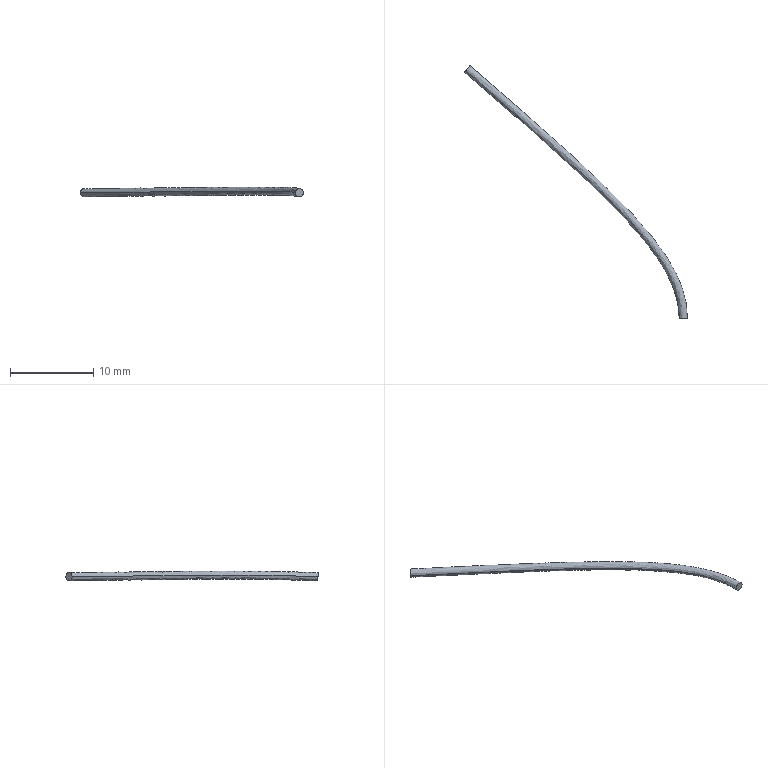Part | NX | features BREP 1 | 1 solid | 4 faces | box 26.795 x 30.33 x 1.202 mm | volume 31.795 mm3 | plane 2 | spline 2
STEP:
#1=CARTESIAN_POINT('',(-445.099,275.62,219.465));
#2=VERTEX_POINT('',#1);
#3=CARTESIAN_POINT('',(-444.445,276.376,219.465));
#4=VERTEX_POINT('',#3);
#5=CARTESIAN_POINT('',(-445.099,275.62,219.465));
#6=CARTESIAN_POINT('',(-445.099,275.62,219.407));
#7=CARTESIAN_POINT('',(-445.084,275.635,219.284));
#8=CARTESIAN_POINT('',(-445.015,275.712,219.115));
#9=CARTESIAN_POINT('',(-444.904,275.838,218.994));
#10=CARTESIAN_POINT('',(-444.769,275.994,218.95));
#11=CARTESIAN_POINT('',(-444.634,276.151,218.994));
#12=CARTESIAN_POINT('',(-444.524,276.279,219.114));
#13=CARTESIAN_POINT('',(-444.457,276.359,219.283));
#14=CARTESIAN_POINT('',(-444.444,276.376,219.406));
#15=CARTESIAN_POINT('',(-444.445,276.376,219.465));
#16=B_SPLINE_CURVE_WITH_KNOTS('',3,(#5,#6,#7,#8,#9,#10,#11,#12,#13,#14,#15),.UNSPECIFIED.,.F.,.F.,(4,1,1,1,1,1,1,1,4),(0.,0.125,0.25,0.375,0.5,0.625,0.75,0.875,1.),.UNSPECIFIED.);
#17=EDGE_CURVE('',#2,#4,#16,.T.);
#18=ORIENTED_EDGE('',*,*,#17,.F.);
#19=CARTESIAN_POINT('',(-444.445,276.376,219.465));
#20=CARTESIAN_POINT('',(-444.445,276.376,219.523));
#21=CARTESIAN_POINT('',(-444.46,276.361,219.646));
#22=CARTESIAN_POINT('',(-444.529,276.284,219.815));
#23=CARTESIAN_POINT('',(-444.64,276.158,219.936));
#24=CARTESIAN_POINT('',(-444.775,276.002,219.98));
#25=CARTESIAN_POINT('',(-444.91,275.845,219.936));
#26=CARTESIAN_POINT('',(-445.02,275.717,219.816));
#27=CARTESIAN_POINT('',(-445.087,275.637,219.647));
#28=CARTESIAN_POINT('',(-445.1,275.62,219.524));
#29=CARTESIAN_POINT('',(-445.099,275.62,219.465));
#30=B_SPLINE_CURVE_WITH_KNOTS('',3,(#19,#20,#21,#22,#23,#24,#25,#26,#27,#28,#29),.UNSPECIFIED.,.F.,.F.,(4,1,1,1,1,1,1,1,4),(0.,0.125,0.25,0.375,0.5,0.625,0.75,0.875,1.),.UNSPECIFIED.);
#31=EDGE_CURVE('',#4,#2,#30,.T.);
#32=ORIENTED_EDGE('',*,*,#31,.F.);
#33=EDGE_LOOP('',(#18,#32));
#34=FACE_BOUND('',#33,.T.);
#35=CARTESIAN_POINT('',(-444.772,275.998,219.465));
#36=DIRECTION('',(-0.7561,0.6544,-0.009303));
#37=DIRECTION('',(0.0123,0.,-0.9999));
#38=AXIS2_PLACEMENT_3D('',#35,#36,#37);
#39=PLANE('',#38);
#40=ADVANCED_FACE('',(#34),#39,.T.);
#41=CARTESIAN_POINT('',(-419.304,246.065,219.473));
#42=VERTEX_POINT('',#41);
#43=CARTESIAN_POINT('',(-419.304,246.065,219.473));
#44=CARTESIAN_POINT('',(-419.307,246.657,219.498));
#45=CARTESIAN_POINT('',(-419.424,247.84,219.543));
#46=CARTESIAN_POINT('',(-419.911,249.573,219.593));
#47=CARTESIAN_POINT('',(-420.651,251.235,219.628));
#48=CARTESIAN_POINT('',(-421.918,253.399,219.658));
#49=CARTESIAN_POINT('',(-423.879,255.957,219.671));
#50=CARTESIAN_POINT('',(-426.566,258.888,219.664));
#51=CARTESIAN_POINT('',(-428.953,261.245,219.647));
#52=CARTESIAN_POINT('',(-430.933,263.114,219.629));
#53=CARTESIAN_POINT('',(-432.476,264.537,219.614));
#54=CARTESIAN_POINT('',(-434.074,265.981,219.597));
#55=CARTESIAN_POINT('',(-436.204,267.878,219.573));
#56=CARTESIAN_POINT('',(-438.731,270.092,219.543));
#57=CARTESIAN_POINT('',(-441.269,272.297,219.512));
#58=CARTESIAN_POINT('',(-443.427,274.171,219.486));
#59=CARTESIAN_POINT('',(-444.541,275.137,219.472));
#60=CARTESIAN_POINT('',(-445.099,275.62,219.465));
#61=B_SPLINE_CURVE_WITH_KNOTS('',3,(#43,#44,#45,#46,#47,#48,#49,#50,#51,#52,#53,#54,#55,#56,#57,#58,#59,#60),.UNSPECIFIED.,.F.,.F.,(4,1,1,1,1,1,1,1,1,1,1,1,1,1,1,4),(0.,0.04528,0.09056,0.1358,0.1811,0.277,0.3729,0.472,0.5215,0.5711,0.6247,0.6783,0.7855,0.8928,0.9464,1.),.UNSPECIFIED.);
#62=EDGE_CURVE('',#42,#2,#61,.T.);
#63=ORIENTED_EDGE('',*,*,#62,.T.);
#64=ORIENTED_EDGE('',*,*,#17,.T.);
#65=CARTESIAN_POINT('',(-418.304,246.071,219.457));
#66=VERTEX_POINT('',#65);
#67=CARTESIAN_POINT('',(-418.304,246.071,219.457));
#68=CARTESIAN_POINT('',(-418.307,246.724,219.485));
#69=CARTESIAN_POINT('',(-418.437,248.031,219.534));
#70=CARTESIAN_POINT('',(-418.968,249.919,219.589));
#71=CARTESIAN_POINT('',(-419.762,251.697,219.626));
#72=CARTESIAN_POINT('',(-421.096,253.973,219.658));
#73=CARTESIAN_POINT('',(-423.118,256.607,219.671));
#74=CARTESIAN_POINT('',(-425.849,259.585,219.663));
#75=CARTESIAN_POINT('',(-428.259,261.964,219.646));
#76=CARTESIAN_POINT('',(-430.251,263.845,219.629));
#77=CARTESIAN_POINT('',(-431.802,265.276,219.613));
#78=CARTESIAN_POINT('',(-433.406,266.725,219.596));
#79=CARTESIAN_POINT('',(-435.543,268.629,219.572));
#80=CARTESIAN_POINT('',(-438.075,270.846,219.542));
#81=CARTESIAN_POINT('',(-440.613,273.052,219.511));
#82=CARTESIAN_POINT('',(-442.771,274.926,219.485));
#83=CARTESIAN_POINT('',(-443.886,275.892,219.471));
#84=CARTESIAN_POINT('',(-444.445,276.376,219.465));
#85=B_SPLINE_CURVE_WITH_KNOTS('',3,(#67,#68,#69,#70,#71,#72,#73,#74,#75,#76,#77,#78,#79,#80,#81,#82,#83,#84),.UNSPECIFIED.,.F.,.F.,(4,1,1,1,1,1,1,1,1,1,1,1,1,1,1,4),(0.,0.04528,0.09056,0.1358,0.1811,0.277,0.3729,0.472,0.5215,0.5711,0.6247,0.6783,0.7855,0.8928,0.9464,1.),.UNSPECIFIED.);
#86=EDGE_CURVE('',#66,#4,#85,.T.);
#87=ORIENTED_EDGE('',*,*,#86,.F.);
#88=CARTESIAN_POINT('',(-419.304,246.065,219.473));
#89=CARTESIAN_POINT('',(-419.305,246.068,219.414));
#90=CARTESIAN_POINT('',(-419.286,246.073,219.292));
#91=CARTESIAN_POINT('',(-419.185,246.081,219.121));
#92=CARTESIAN_POINT('',(-419.019,246.087,218.998));
#93=CARTESIAN_POINT('',(-418.812,246.09,218.951));
#94=CARTESIAN_POINT('',(-418.605,246.089,218.991));
#95=CARTESIAN_POINT('',(-418.434,246.085,219.109));
#96=CARTESIAN_POINT('',(-418.328,246.078,219.276));
#97=CARTESIAN_POINT('',(-418.305,246.073,219.398));
#98=CARTESIAN_POINT('',(-418.304,246.071,219.457));
#99=B_SPLINE_CURVE_WITH_KNOTS('',3,(#88,#89,#90,#91,#92,#93,#94,#95,#96,#97,#98),.UNSPECIFIED.,.F.,.F.,(4,1,1,1,1,1,1,1,4),(0.,0.125,0.25,0.375,0.5,0.625,0.75,0.875,1.),.UNSPECIFIED.);
#100=EDGE_CURVE('',#42,#66,#99,.T.);
#101=ORIENTED_EDGE('',*,*,#100,.F.);
#102=EDGE_LOOP('',(#63,#64,#87,#101));
#103=FACE_BOUND('',#102,.T.);
#104=CARTESIAN_POINT('',(-444.445,276.376,219.465));
#105=CARTESIAN_POINT('',(-444.444,276.376,219.406));
#106=CARTESIAN_POINT('',(-444.457,276.359,219.283));
#107=CARTESIAN_POINT('',(-444.524,276.279,219.114));
#108=CARTESIAN_POINT('',(-444.634,276.151,218.994));
#109=CARTESIAN_POINT('',(-444.769,275.994,218.95));
#110=CARTESIAN_POINT('',(-444.904,275.838,218.994));
#111=CARTESIAN_POINT('',(-445.015,275.712,219.115));
#112=CARTESIAN_POINT('',(-445.084,275.635,219.284));
#113=CARTESIAN_POINT('',(-445.099,275.62,219.407));
#114=CARTESIAN_POINT('',(-445.099,275.62,219.465));
#115=CARTESIAN_POINT('',(-443.886,275.892,219.471));
#116=CARTESIAN_POINT('',(-443.886,275.892,219.412));
#117=CARTESIAN_POINT('',(-443.899,275.875,219.29));
#118=CARTESIAN_POINT('',(-443.965,275.796,219.121));
#119=CARTESIAN_POINT('',(-444.075,275.668,219.001));
#120=CARTESIAN_POINT('',(-444.21,275.511,218.957));
#121=CARTESIAN_POINT('',(-444.346,275.355,219.001));
#122=CARTESIAN_POINT('',(-444.457,275.229,219.122));
#123=CARTESIAN_POINT('',(-444.526,275.151,219.291));
#124=CARTESIAN_POINT('',(-444.541,275.136,219.413));
#125=CARTESIAN_POINT('',(-444.541,275.137,219.472));
#126=CARTESIAN_POINT('',(-442.771,274.926,219.485));
#127=CARTESIAN_POINT('',(-442.771,274.925,219.426));
#128=CARTESIAN_POINT('',(-442.784,274.909,219.304));
#129=CARTESIAN_POINT('',(-442.851,274.829,219.135));
#130=CARTESIAN_POINT('',(-442.96,274.701,219.015));
#131=CARTESIAN_POINT('',(-443.096,274.545,218.971));
#132=CARTESIAN_POINT('',(-443.232,274.389,219.015));
#133=CARTESIAN_POINT('',(-443.343,274.262,219.136));
#134=CARTESIAN_POINT('',(-443.412,274.185,219.305));
#135=CARTESIAN_POINT('',(-443.426,274.17,219.427));
#136=CARTESIAN_POINT('',(-443.427,274.171,219.486));
#137=CARTESIAN_POINT('',(-440.613,273.052,219.511));
#138=CARTESIAN_POINT('',(-440.613,273.052,219.452));
#139=CARTESIAN_POINT('',(-440.626,273.035,219.33));
#140=CARTESIAN_POINT('',(-440.693,272.956,219.161));
#141=CARTESIAN_POINT('',(-440.803,272.828,219.041));
#142=CARTESIAN_POINT('',(-440.938,272.671,218.997));
#143=CARTESIAN_POINT('',(-441.074,272.515,219.041));
#144=CARTESIAN_POINT('',(-441.185,272.389,219.162));
#145=CARTESIAN_POINT('',(-441.254,272.312,219.331));
#146=CARTESIAN_POINT('',(-441.269,272.297,219.453));
#147=CARTESIAN_POINT('',(-441.269,272.297,219.512));
#148=CARTESIAN_POINT('',(-438.075,270.846,219.542));
#149=CARTESIAN_POINT('',(-438.074,270.846,219.483));
#150=CARTESIAN_POINT('',(-438.088,270.829,219.361));
#151=CARTESIAN_POINT('',(-438.155,270.75,219.192));
#152=CARTESIAN_POINT('',(-438.264,270.622,219.072));
#153=CARTESIAN_POINT('',(-438.4,270.466,219.028));
#154=CARTESIAN_POINT('',(-438.536,270.31,219.072));
#155=CARTESIAN_POINT('',(-438.647,270.184,219.193));
#156=CARTESIAN_POINT('',(-438.716,270.107,219.362));
#157=CARTESIAN_POINT('',(-438.731,270.092,219.484));
#158=CARTESIAN_POINT('',(-438.731,270.092,219.543));
#159=CARTESIAN_POINT('',(-435.543,268.629,219.572));
#160=CARTESIAN_POINT('',(-435.543,268.628,219.513));
#161=CARTESIAN_POINT('',(-435.556,268.612,219.391));
#162=CARTESIAN_POINT('',(-435.623,268.533,219.222));
#163=CARTESIAN_POINT('',(-435.734,268.406,219.102));
#164=CARTESIAN_POINT('',(-435.87,268.25,219.058));
#165=CARTESIAN_POINT('',(-436.008,268.095,219.102));
#166=CARTESIAN_POINT('',(-436.12,267.97,219.223));
#167=CARTESIAN_POINT('',(-436.189,267.893,219.392));
#168=CARTESIAN_POINT('',(-436.204,267.878,219.514));
#169=CARTESIAN_POINT('',(-436.204,267.878,219.573));
#170=CARTESIAN_POINT('',(-433.406,266.725,219.596));
#171=CARTESIAN_POINT('',(-433.406,266.725,219.537));
#172=CARTESIAN_POINT('',(-433.419,266.709,219.415));
#173=CARTESIAN_POINT('',(-433.487,266.63,219.246));
#174=CARTESIAN_POINT('',(-433.599,266.504,219.126));
#175=CARTESIAN_POINT('',(-433.737,266.35,219.082));
#176=CARTESIAN_POINT('',(-433.875,266.196,219.126));
#177=CARTESIAN_POINT('',(-433.988,266.072,219.247));
#178=CARTESIAN_POINT('',(-434.058,265.995,219.416));
#179=CARTESIAN_POINT('',(-434.073,265.98,219.538));
#180=CARTESIAN_POINT('',(-434.074,265.981,219.597));
#181=CARTESIAN_POINT('',(-431.802,265.276,219.613));
#182=CARTESIAN_POINT('',(-431.802,265.275,219.554));
#183=CARTESIAN_POINT('',(-431.816,265.259,219.432));
#184=CARTESIAN_POINT('',(-431.885,265.182,219.263));
#185=CARTESIAN_POINT('',(-431.998,265.057,219.143));
#186=CARTESIAN_POINT('',(-432.137,264.903,219.099));
#187=CARTESIAN_POINT('',(-432.277,264.751,219.143));
#188=CARTESIAN_POINT('',(-432.391,264.627,219.264));
#189=CARTESIAN_POINT('',(-432.461,264.551,219.433));
#190=CARTESIAN_POINT('',(-432.476,264.536,219.555));
#191=CARTESIAN_POINT('',(-432.476,264.537,219.614));
#192=CARTESIAN_POINT('',(-430.251,263.845,219.629));
#193=CARTESIAN_POINT('',(-430.251,263.845,219.57));
#194=CARTESIAN_POINT('',(-430.265,263.829,219.447));
#195=CARTESIAN_POINT('',(-430.334,263.752,219.278));
#196=CARTESIAN_POINT('',(-430.449,263.629,219.158));
#197=CARTESIAN_POINT('',(-430.59,263.477,219.114));
#198=CARTESIAN_POINT('',(-430.731,263.326,219.158));
#199=CARTESIAN_POINT('',(-430.846,263.203,219.279));
#200=CARTESIAN_POINT('',(-430.918,263.128,219.448));
#201=CARTESIAN_POINT('',(-430.933,263.114,219.57));
#202=CARTESIAN_POINT('',(-430.933,263.114,219.629));
#203=CARTESIAN_POINT('',(-428.259,261.964,219.646));
#204=CARTESIAN_POINT('',(-428.258,261.964,219.587));
#205=CARTESIAN_POINT('',(-428.273,261.948,219.465));
#206=CARTESIAN_POINT('',(-428.344,261.873,219.296));
#207=CARTESIAN_POINT('',(-428.46,261.751,219.176));
#208=CARTESIAN_POINT('',(-428.604,261.602,219.132));
#209=CARTESIAN_POINT('',(-428.748,261.454,219.176));
#210=CARTESIAN_POINT('',(-428.865,261.333,219.297));
#211=CARTESIAN_POINT('',(-428.938,261.259,219.466));
#212=CARTESIAN_POINT('',(-428.953,261.245,219.588));
#213=CARTESIAN_POINT('',(-428.953,261.245,219.647));
#214=CARTESIAN_POINT('',(-425.849,259.585,219.663));
#215=CARTESIAN_POINT('',(-425.849,259.585,219.605));
#216=CARTESIAN_POINT('',(-425.864,259.57,219.482));
#217=CARTESIAN_POINT('',(-425.938,259.497,219.313));
#218=CARTESIAN_POINT('',(-426.058,259.379,219.193));
#219=CARTESIAN_POINT('',(-426.206,259.235,219.149));
#220=CARTESIAN_POINT('',(-426.355,259.091,219.193));
#221=CARTESIAN_POINT('',(-426.476,258.974,219.313));
#222=CARTESIAN_POINT('',(-426.55,258.902,219.482));
#223=CARTESIAN_POINT('',(-426.566,258.887,219.605));
#224=CARTESIAN_POINT('',(-426.566,258.888,219.664));
#225=CARTESIAN_POINT('',(-423.118,256.607,219.671));
#226=CARTESIAN_POINT('',(-423.118,256.607,219.612));
#227=CARTESIAN_POINT('',(-423.135,256.593,219.489));
#228=CARTESIAN_POINT('',(-423.213,256.526,219.32));
#229=CARTESIAN_POINT('',(-423.342,256.417,219.2));
#230=CARTESIAN_POINT('',(-423.499,256.282,219.156));
#231=CARTESIAN_POINT('',(-423.657,256.147,219.2));
#232=CARTESIAN_POINT('',(-423.785,256.038,219.321));
#233=CARTESIAN_POINT('',(-423.863,255.971,219.49));
#234=CARTESIAN_POINT('',(-423.879,255.957,219.612));
#235=CARTESIAN_POINT('',(-423.879,255.957,219.671));
#236=CARTESIAN_POINT('',(-421.096,253.973,219.658));
#237=CARTESIAN_POINT('',(-421.096,253.973,219.599));
#238=CARTESIAN_POINT('',(-421.114,253.962,219.476));
#239=CARTESIAN_POINT('',(-421.2,253.903,219.307));
#240=CARTESIAN_POINT('',(-421.339,253.807,219.187));
#241=CARTESIAN_POINT('',(-421.509,253.689,219.143));
#242=CARTESIAN_POINT('',(-421.679,253.57,219.187));
#243=CARTESIAN_POINT('',(-421.817,253.472,219.308));
#244=CARTESIAN_POINT('',(-421.901,253.412,219.477));
#245=CARTESIAN_POINT('',(-421.918,253.399,219.599));
#246=CARTESIAN_POINT('',(-421.918,253.399,219.658));
#247=CARTESIAN_POINT('',(-419.762,251.697,219.626));
#248=CARTESIAN_POINT('',(-419.762,251.698,219.567));
#249=CARTESIAN_POINT('',(-419.782,251.69,219.445));
#250=CARTESIAN_POINT('',(-419.876,251.644,219.276));
#251=CARTESIAN_POINT('',(-420.027,251.568,219.156));
#252=CARTESIAN_POINT('',(-420.211,251.473,219.113));
#253=CARTESIAN_POINT('',(-420.395,251.376,219.157));
#254=CARTESIAN_POINT('',(-420.543,251.297,219.277));
#255=CARTESIAN_POINT('',(-420.634,251.247,219.447));
#256=CARTESIAN_POINT('',(-420.651,251.236,219.569));
#257=CARTESIAN_POINT('',(-420.651,251.235,219.628));
#258=CARTESIAN_POINT('',(-418.968,249.919,219.589));
#259=CARTESIAN_POINT('',(-418.969,249.92,219.53));
#260=CARTESIAN_POINT('',(-418.991,249.915,219.408));
#261=CARTESIAN_POINT('',(-419.09,249.883,219.239));
#262=CARTESIAN_POINT('',(-419.251,249.827,219.12));
#263=CARTESIAN_POINT('',(-419.446,249.756,219.077));
#264=CARTESIAN_POINT('',(-419.641,249.684,219.121));
#265=CARTESIAN_POINT('',(-419.798,249.623,219.243));
#266=CARTESIAN_POINT('',(-419.894,249.584,219.412));
#267=CARTESIAN_POINT('',(-419.912,249.574,219.534));
#268=CARTESIAN_POINT('',(-419.911,249.573,219.593));
#269=CARTESIAN_POINT('',(-418.437,248.031,219.534));
#270=CARTESIAN_POINT('',(-418.438,248.032,219.475));
#271=CARTESIAN_POINT('',(-418.461,248.032,219.353));
#272=CARTESIAN_POINT('',(-418.566,248.017,219.185));
#273=CARTESIAN_POINT('',(-418.734,247.989,219.066));
#274=CARTESIAN_POINT('',(-418.939,247.951,219.024));
#275=CARTESIAN_POINT('',(-419.142,247.91,219.07));
#276=CARTESIAN_POINT('',(-419.306,247.875,219.192));
#277=CARTESIAN_POINT('',(-419.406,247.85,219.362));
#278=CARTESIAN_POINT('',(-419.425,247.842,219.484));
#279=CARTESIAN_POINT('',(-419.424,247.84,219.543));
#280=CARTESIAN_POINT('',(-418.307,246.724,219.485));
#281=CARTESIAN_POINT('',(-418.308,246.727,219.426));
#282=CARTESIAN_POINT('',(-418.331,246.73,219.304));
#283=CARTESIAN_POINT('',(-418.438,246.729,219.136));
#284=CARTESIAN_POINT('',(-418.608,246.723,219.018));
#285=CARTESIAN_POINT('',(-418.816,246.711,218.977));
#286=CARTESIAN_POINT('',(-419.022,246.695,219.024));
#287=CARTESIAN_POINT('',(-419.188,246.679,219.147));
#288=CARTESIAN_POINT('',(-419.289,246.665,219.317));
#289=CARTESIAN_POINT('',(-419.308,246.659,219.439));
#290=CARTESIAN_POINT('',(-419.307,246.657,219.498));
#291=CARTESIAN_POINT('',(-418.304,246.071,219.457));
#292=CARTESIAN_POINT('',(-418.305,246.073,219.398));
#293=CARTESIAN_POINT('',(-418.328,246.078,219.276));
#294=CARTESIAN_POINT('',(-418.434,246.085,219.109));
#295=CARTESIAN_POINT('',(-418.605,246.089,218.991));
#296=CARTESIAN_POINT('',(-418.812,246.09,218.951));
#297=CARTESIAN_POINT('',(-419.019,246.087,218.998));
#298=CARTESIAN_POINT('',(-419.185,246.081,219.121));
#299=CARTESIAN_POINT('',(-419.286,246.073,219.292));
#300=CARTESIAN_POINT('',(-419.305,246.068,219.414));
#301=CARTESIAN_POINT('',(-419.304,246.065,219.473));
#302=B_SPLINE_SURFACE_WITH_KNOTS('',3,3,((#104,#105,#106,#107,#108,#109,#110,#111,#112,#113,#114),(#115,#116,#117,#118,#119,#120,#121,#122,#123,#124,#125),(#126,#127,#128,#129,#130,#131,#132,#133,#134,#135,#136),(#137,#138,#139,#140,#141,#142,#143,#144,#145,#146,#147),(#148,#149,#150,#151,#152,#153,#154,#155,#156,#157,#158),(#159,#160,#161,#162,#163,#164,#165,#166,#167,#168,#169),(#170,#171,#172,#173,#174,#175,#176,#177,#178,#179,#180),(#181,#182,#183,#184,#185,#186,#187,#188,#189,#190,#191),(#192,#193,#194,#195,#196,#197,#198,#199,#200,#201,#202),(#203,#204,#205,#206,#207,#208,#209,#210,#211,#212,#213),(#214,#215,#216,#217,#218,#219,#220,#221,#222,#223,#224),(#225,#226,#227,#228,#229,#230,#231,#232,#233,#234,#235),(#236,#237,#238,#239,#240,#241,#242,#243,#244,#245,#246),(#247,#248,#249,#250,#251,#252,#253,#254,#255,#256,#257),(#258,#259,#260,#261,#262,#263,#264,#265,#266,#267,#268),(#269,#270,#271,#272,#273,#274,#275,#276,#277,#278,#279),(#280,#281,#282,#283,#284,#285,#286,#287,#288,#289,#290),(#291,#292,#293,#294,#295,#296,#297,#298,#299,#300,#301)),.UNSPECIFIED.,.F.,.F.,.F.,(4,1,1,1,1,1,1,1,1,1,1,1,1,1,1,4),(4,1,1,1,1,1,1,1,4),(0.009511,0.06212,0.1147,0.2199,0.3252,0.3778,0.4304,0.479,0.5276,0.6248,0.7189,0.813,0.8574,0.9019,0.9463,0.9907),(0.01855,0.1389,0.2593,0.3797,0.5001,0.6205,0.7409,0.8613,0.9817),.UNSPECIFIED.);
#303=ADVANCED_FACE('',(#103),#302,.T.);
#304=ORIENTED_EDGE('',*,*,#86,.T.);
#305=ORIENTED_EDGE('',*,*,#31,.T.);
#306=ORIENTED_EDGE('',*,*,#62,.F.);
#307=CARTESIAN_POINT('',(-418.304,246.071,219.457));
#308=CARTESIAN_POINT('',(-418.303,246.068,219.516));
#309=CARTESIAN_POINT('',(-418.322,246.063,219.638));
#310=CARTESIAN_POINT('',(-418.423,246.055,219.809));
#311=CARTESIAN_POINT('',(-418.589,246.049,219.932));
#312=CARTESIAN_POINT('',(-418.796,246.046,219.979));
#313=CARTESIAN_POINT('',(-419.003,246.047,219.939));
#314=CARTESIAN_POINT('',(-419.174,246.051,219.821));
#315=CARTESIAN_POINT('',(-419.28,246.058,219.654));
#316=CARTESIAN_POINT('',(-419.303,246.063,219.532));
#317=CARTESIAN_POINT('',(-419.304,246.065,219.473));
#318=B_SPLINE_CURVE_WITH_KNOTS('',3,(#307,#308,#309,#310,#311,#312,#313,#314,#315,#316,#317),.UNSPECIFIED.,.F.,.F.,(4,1,1,1,1,1,1,1,4),(0.,0.125,0.25,0.375,0.5,0.625,0.75,0.875,1.),.UNSPECIFIED.);
#319=EDGE_CURVE('',#66,#42,#318,.T.);
#320=ORIENTED_EDGE('',*,*,#319,.F.);
#321=EDGE_LOOP('',(#304,#305,#306,#320));
#322=FACE_BOUND('',#321,.T.);
#323=CARTESIAN_POINT('',(-445.099,275.62,219.465));
#324=CARTESIAN_POINT('',(-445.1,275.62,219.524));
#325=CARTESIAN_POINT('',(-445.087,275.637,219.647));
#326=CARTESIAN_POINT('',(-445.02,275.717,219.816));
#327=CARTESIAN_POINT('',(-444.91,275.845,219.936));
#328=CARTESIAN_POINT('',(-444.775,276.002,219.98));
#329=CARTESIAN_POINT('',(-444.64,276.158,219.936));
#330=CARTESIAN_POINT('',(-444.529,276.284,219.815));
#331=CARTESIAN_POINT('',(-444.46,276.361,219.646));
#332=CARTESIAN_POINT('',(-444.445,276.376,219.523));
#333=CARTESIAN_POINT('',(-444.445,276.376,219.465));
#334=CARTESIAN_POINT('',(-444.541,275.137,219.472));
#335=CARTESIAN_POINT('',(-444.541,275.137,219.531));
#336=CARTESIAN_POINT('',(-444.528,275.154,219.654));
#337=CARTESIAN_POINT('',(-444.461,275.233,219.823));
#338=CARTESIAN_POINT('',(-444.352,275.361,219.943));
#339=CARTESIAN_POINT('',(-444.217,275.518,219.986));
#340=CARTESIAN_POINT('',(-444.081,275.674,219.942));
#341=CARTESIAN_POINT('',(-443.97,275.801,219.822));
#342=CARTESIAN_POINT('',(-443.901,275.878,219.653));
#343=CARTESIAN_POINT('',(-443.886,275.893,219.53));
#344=CARTESIAN_POINT('',(-443.886,275.892,219.471));
#345=CARTESIAN_POINT('',(-443.427,274.171,219.486));
#346=CARTESIAN_POINT('',(-443.427,274.171,219.545));
#347=CARTESIAN_POINT('',(-443.414,274.188,219.667));
#348=CARTESIAN_POINT('',(-443.347,274.267,219.836));
#349=CARTESIAN_POINT('',(-443.238,274.395,219.956));
#350=CARTESIAN_POINT('',(-443.102,274.552,220.));
#351=CARTESIAN_POINT('',(-442.966,274.708,219.956));
#352=CARTESIAN_POINT('',(-442.855,274.834,219.835));
#353=CARTESIAN_POINT('',(-442.786,274.911,219.666));
#354=CARTESIAN_POINT('',(-442.772,274.926,219.544));
#355=CARTESIAN_POINT('',(-442.771,274.926,219.485));
#356=CARTESIAN_POINT('',(-441.269,272.297,219.512));
#357=CARTESIAN_POINT('',(-441.269,272.298,219.571));
#358=CARTESIAN_POINT('',(-441.256,272.314,219.694));
#359=CARTESIAN_POINT('',(-441.189,272.394,219.862));
#360=CARTESIAN_POINT('',(-441.08,272.522,219.983));
#361=CARTESIAN_POINT('',(-440.944,272.678,220.026));
#362=CARTESIAN_POINT('',(-440.808,272.834,219.982));
#363=CARTESIAN_POINT('',(-440.697,272.96,219.862));
#364=CARTESIAN_POINT('',(-440.628,273.038,219.693));
#365=CARTESIAN_POINT('',(-440.614,273.053,219.57));
#366=CARTESIAN_POINT('',(-440.613,273.052,219.511));
#367=CARTESIAN_POINT('',(-438.731,270.092,219.543));
#368=CARTESIAN_POINT('',(-438.732,270.092,219.602));
#369=CARTESIAN_POINT('',(-438.719,270.109,219.724));
#370=CARTESIAN_POINT('',(-438.652,270.188,219.893));
#371=CARTESIAN_POINT('',(-438.542,270.316,220.014));
#372=CARTESIAN_POINT('',(-438.406,270.473,220.057));
#373=CARTESIAN_POINT('',(-438.27,270.629,220.013));
#374=CARTESIAN_POINT('',(-438.159,270.755,219.893));
#375=CARTESIAN_POINT('',(-438.09,270.832,219.724));
#376=CARTESIAN_POINT('',(-438.075,270.847,219.601));
#377=CARTESIAN_POINT('',(-438.075,270.846,219.542));
#378=CARTESIAN_POINT('',(-436.204,267.878,219.573));
#379=CARTESIAN_POINT('',(-436.204,267.879,219.632));
#380=CARTESIAN_POINT('',(-436.191,267.895,219.754));
#381=CARTESIAN_POINT('',(-436.124,267.974,219.923));
#382=CARTESIAN_POINT('',(-436.013,268.101,220.044));
#383=CARTESIAN_POINT('',(-435.877,268.257,220.087));
#384=CARTESIAN_POINT('',(-435.739,268.412,220.043));
#385=CARTESIAN_POINT('',(-435.628,268.537,219.923));
#386=CARTESIAN_POINT('',(-435.558,268.614,219.754));
#387=CARTESIAN_POINT('',(-435.543,268.629,219.631));
#388=CARTESIAN_POINT('',(-435.543,268.629,219.572));
#389=CARTESIAN_POINT('',(-434.074,265.981,219.597));
#390=CARTESIAN_POINT('',(-434.074,265.981,219.656));
#391=CARTESIAN_POINT('',(-434.06,265.998,219.778));
#392=CARTESIAN_POINT('',(-433.992,266.076,219.947));
#393=CARTESIAN_POINT('',(-433.881,266.202,220.068));
#394=CARTESIAN_POINT('',(-433.743,266.356,220.111));
#395=CARTESIAN_POINT('',(-433.604,266.51,220.067));
#396=CARTESIAN_POINT('',(-433.491,266.635,219.947));
#397=CARTESIAN_POINT('',(-433.421,266.711,219.778));
#398=CARTESIAN_POINT('',(-433.406,266.726,219.655));
#399=CARTESIAN_POINT('',(-433.406,266.725,219.596));
#400=CARTESIAN_POINT('',(-432.476,264.537,219.614));
#401=CARTESIAN_POINT('',(-432.477,264.537,219.673));
#402=CARTESIAN_POINT('',(-432.463,264.553,219.795));
#403=CARTESIAN_POINT('',(-432.394,264.631,219.964));
#404=CARTESIAN_POINT('',(-432.281,264.756,220.085));
#405=CARTESIAN_POINT('',(-432.142,264.909,220.128));
#406=CARTESIAN_POINT('',(-432.002,265.062,220.084));
#407=CARTESIAN_POINT('',(-431.888,265.186,219.964));
#408=CARTESIAN_POINT('',(-431.818,265.261,219.795));
#409=CARTESIAN_POINT('',(-431.803,265.276,219.672));
#410=CARTESIAN_POINT('',(-431.802,265.276,219.613));
#411=CARTESIAN_POINT('',(-430.933,263.114,219.629));
#412=CARTESIAN_POINT('',(-430.933,263.114,219.688));
#413=CARTESIAN_POINT('',(-430.919,263.13,219.811));
#414=CARTESIAN_POINT('',(-430.849,263.207,219.979));
#415=CARTESIAN_POINT('',(-430.735,263.331,220.1));
#416=CARTESIAN_POINT('',(-430.594,263.482,220.144));
#417=CARTESIAN_POINT('',(-430.453,263.634,220.1));
#418=CARTESIAN_POINT('',(-430.338,263.756,219.979));
#419=CARTESIAN_POINT('',(-430.266,263.831,219.81));
#420=CARTESIAN_POINT('',(-430.251,263.846,219.688));
#421=CARTESIAN_POINT('',(-430.251,263.845,219.629));
#422=CARTESIAN_POINT('',(-428.953,261.245,219.647));
#423=CARTESIAN_POINT('',(-428.954,261.245,219.706));
#424=CARTESIAN_POINT('',(-428.939,261.261,219.828));
#425=CARTESIAN_POINT('',(-428.868,261.336,219.997));
#426=CARTESIAN_POINT('',(-428.752,261.458,220.118));
#427=CARTESIAN_POINT('',(-428.608,261.607,220.161));
#428=CARTESIAN_POINT('',(-428.464,261.756,220.117));
#429=CARTESIAN_POINT('',(-428.347,261.876,219.997));
#430=CARTESIAN_POINT('',(-428.274,261.95,219.828));
#431=CARTESIAN_POINT('',(-428.259,261.964,219.705));
#432=CARTESIAN_POINT('',(-428.259,261.964,219.646));
#433=CARTESIAN_POINT('',(-426.566,258.888,219.664));
#434=CARTESIAN_POINT('',(-426.566,258.888,219.723));
#435=CARTESIAN_POINT('',(-426.551,258.903,219.845));
#436=CARTESIAN_POINT('',(-426.477,258.976,220.014));
#437=CARTESIAN_POINT('',(-426.357,259.093,220.134));
#438=CARTESIAN_POINT('',(-426.209,259.238,220.178));
#439=CARTESIAN_POINT('',(-426.06,259.382,220.134));
#440=CARTESIAN_POINT('',(-425.939,259.499,220.014));
#441=CARTESIAN_POINT('',(-425.865,259.571,219.845));
#442=CARTESIAN_POINT('',(-425.849,259.585,219.722));
#443=CARTESIAN_POINT('',(-425.849,259.585,219.663));
#444=CARTESIAN_POINT('',(-423.879,255.957,219.671));
#445=CARTESIAN_POINT('',(-423.879,255.957,219.73));
#446=CARTESIAN_POINT('',(-423.863,255.97,219.852));
#447=CARTESIAN_POINT('',(-423.784,256.038,220.021));
#448=CARTESIAN_POINT('',(-423.656,256.147,220.142));
#449=CARTESIAN_POINT('',(-423.499,256.282,220.185));
#450=CARTESIAN_POINT('',(-423.341,256.416,220.142));
#451=CARTESIAN_POINT('',(-423.213,256.526,220.021));
#452=CARTESIAN_POINT('',(-423.134,256.593,219.852));
#453=CARTESIAN_POINT('',(-423.118,256.607,219.73));
#454=CARTESIAN_POINT('',(-423.118,256.607,219.671));
#455=CARTESIAN_POINT('',(-421.918,253.399,219.658));
#456=CARTESIAN_POINT('',(-421.918,253.399,219.717));
#457=CARTESIAN_POINT('',(-421.9,253.41,219.84));
#458=CARTESIAN_POINT('',(-421.814,253.469,220.008));
#459=CARTESIAN_POINT('',(-421.675,253.565,220.129));
#460=CARTESIAN_POINT('',(-421.504,253.683,220.173));
#461=CARTESIAN_POINT('',(-421.334,253.803,220.129));
#462=CARTESIAN_POINT('',(-421.197,253.9,220.008));
#463=CARTESIAN_POINT('',(-421.112,253.96,219.839));
#464=CARTESIAN_POINT('',(-421.095,253.973,219.717));
#465=CARTESIAN_POINT('',(-421.096,253.973,219.658));
#466=CARTESIAN_POINT('',(-420.651,251.235,219.628));
#467=CARTESIAN_POINT('',(-420.65,251.234,219.687));
#468=CARTESIAN_POINT('',(-420.63,251.242,219.809));
#469=CARTESIAN_POINT('',(-420.537,251.288,219.978));
#470=CARTESIAN_POINT('',(-420.386,251.364,220.098));
#471=CARTESIAN_POINT('',(-420.202,251.46,220.142));
#472=CARTESIAN_POINT('',(-420.018,251.556,220.097));
#473=CARTESIAN_POINT('',(-419.869,251.635,219.977));
#474=CARTESIAN_POINT('',(-419.779,251.685,219.807));
#475=CARTESIAN_POINT('',(-419.761,251.697,219.685));
#476=CARTESIAN_POINT('',(-419.762,251.697,219.626));
#477=CARTESIAN_POINT('',(-419.911,249.573,219.593));
#478=CARTESIAN_POINT('',(-419.911,249.572,219.652));
#479=CARTESIAN_POINT('',(-419.889,249.577,219.775));
#480=CARTESIAN_POINT('',(-419.789,249.609,219.943));
#481=CARTESIAN_POINT('',(-419.629,249.665,220.063));
#482=CARTESIAN_POINT('',(-419.433,249.736,220.106));
#483=CARTESIAN_POINT('',(-419.239,249.808,220.061));
#484=CARTESIAN_POINT('',(-419.082,249.869,219.94));
#485=CARTESIAN_POINT('',(-418.986,249.908,219.77));
#486=CARTESIAN_POINT('',(-418.968,249.918,219.648));
#487=CARTESIAN_POINT('',(-418.968,249.919,219.589));
#488=CARTESIAN_POINT('',(-419.424,247.84,219.543));
#489=CARTESIAN_POINT('',(-419.423,247.838,219.602));
#490=CARTESIAN_POINT('',(-419.401,247.839,219.724));
#491=CARTESIAN_POINT('',(-419.296,247.853,219.892));
#492=CARTESIAN_POINT('',(-419.128,247.882,220.011));
#493=CARTESIAN_POINT('',(-418.923,247.92,220.053));
#494=CARTESIAN_POINT('',(-418.719,247.961,220.007));
#495=CARTESIAN_POINT('',(-418.555,247.996,219.886));
#496=CARTESIAN_POINT('',(-418.455,248.021,219.716));
#497=CARTESIAN_POINT('',(-418.436,248.029,219.593));
#498=CARTESIAN_POINT('',(-418.437,248.031,219.534));
#499=CARTESIAN_POINT('',(-419.307,246.657,219.498));
#500=CARTESIAN_POINT('',(-419.306,246.655,219.557));
#501=CARTESIAN_POINT('',(-419.283,246.652,219.679));
#502=CARTESIAN_POINT('',(-419.177,246.652,219.847));
#503=CARTESIAN_POINT('',(-419.006,246.659,219.965));
#504=CARTESIAN_POINT('',(-418.799,246.671,220.006));
#505=CARTESIAN_POINT('',(-418.593,246.687,219.959));
#506=CARTESIAN_POINT('',(-418.426,246.703,219.837));
#507=CARTESIAN_POINT('',(-418.326,246.716,219.666));
#508=CARTESIAN_POINT('',(-418.306,246.722,219.544));
#509=CARTESIAN_POINT('',(-418.307,246.724,219.485));
#510=CARTESIAN_POINT('',(-419.304,246.065,219.473));
#511=CARTESIAN_POINT('',(-419.303,246.063,219.532));
#512=CARTESIAN_POINT('',(-419.28,246.058,219.654));
#513=CARTESIAN_POINT('',(-419.174,246.051,219.821));
#514=CARTESIAN_POINT('',(-419.003,246.047,219.939));
#515=CARTESIAN_POINT('',(-418.796,246.046,219.979));
#516=CARTESIAN_POINT('',(-418.589,246.049,219.932));
#517=CARTESIAN_POINT('',(-418.423,246.055,219.809));
#518=CARTESIAN_POINT('',(-418.322,246.063,219.638));
#519=CARTESIAN_POINT('',(-418.303,246.068,219.516));
#520=CARTESIAN_POINT('',(-418.304,246.071,219.457));
#521=B_SPLINE_SURFACE_WITH_KNOTS('',3,3,((#323,#324,#325,#326,#327,#328,#329,#330,#331,#332,#333),(#334,#335,#336,#337,#338,#339,#340,#341,#342,#343,#344),(#345,#346,#347,#348,#349,#350,#351,#352,#353,#354,#355),(#356,#357,#358,#359,#360,#361,#362,#363,#364,#365,#366),(#367,#368,#369,#370,#371,#372,#373,#374,#375,#376,#377),(#378,#379,#380,#381,#382,#383,#384,#385,#386,#387,#388),(#389,#390,#391,#392,#393,#394,#395,#396,#397,#398,#399),(#400,#401,#402,#403,#404,#405,#406,#407,#408,#409,#410),(#411,#412,#413,#414,#415,#416,#417,#418,#419,#420,#421),(#422,#423,#424,#425,#426,#427,#428,#429,#430,#431,#432),(#433,#434,#435,#436,#437,#438,#439,#440,#441,#442,#443),(#444,#445,#446,#447,#448,#449,#450,#451,#452,#453,#454),(#455,#456,#457,#458,#459,#460,#461,#462,#463,#464,#465),(#466,#467,#468,#469,#470,#471,#472,#473,#474,#475,#476),(#477,#478,#479,#480,#481,#482,#483,#484,#485,#486,#487),(#488,#489,#490,#491,#492,#493,#494,#495,#496,#497,#498),(#499,#500,#501,#502,#503,#504,#505,#506,#507,#508,#509),(#510,#511,#512,#513,#514,#515,#516,#517,#518,#519,#520)),.UNSPECIFIED.,.F.,.F.,.F.,(4,1,1,1,1,1,1,1,1,1,1,1,1,1,1,4),(4,1,1,1,1,1,1,1,4),(0.009511,0.06212,0.1147,0.2199,0.3252,0.3778,0.4304,0.479,0.5276,0.6248,0.7189,0.813,0.8574,0.9019,0.9463,0.9907),(0.01855,0.1389,0.2593,0.3797,0.5001,0.6205,0.7409,0.8613,0.9817),.UNSPECIFIED.);
#522=ADVANCED_FACE('',(#322),#521,.T.);
#523=ORIENTED_EDGE('',*,*,#319,.T.);
#524=ORIENTED_EDGE('',*,*,#100,.T.);
#525=EDGE_LOOP('',(#523,#524));
#526=FACE_BOUND('',#525,.T.);
#527=CARTESIAN_POINT('',(-418.804,246.068,219.465));
#528=DIRECTION('',(-0.005052,0.9991,0.04256));
#529=DIRECTION('',(-0.993,0.,-0.1179));
#530=AXIS2_PLACEMENT_3D('',#527,#528,#529);
#531=PLANE('',#530);
#532=ADVANCED_FACE('',(#526),#531,.F.);
#533=CLOSED_SHELL('',(#40,#303,#522,#532));
#534=MANIFOLD_SOLID_BREP('',#533);
#535=(LENGTH_UNIT()NAMED_UNIT(*)SI_UNIT(.MILLI.,.METRE.));
#536=UNCERTAINTY_MEASURE_WITH_UNIT(LENGTH_MEASURE(0.00001),#535,'','');
#537=(NAMED_UNIT(*)PLANE_ANGLE_UNIT()SI_UNIT($,.RADIAN.));
#538=(NAMED_UNIT(*)SI_UNIT($,.STERADIAN.)SOLID_ANGLE_UNIT());
#539=(GEOMETRIC_REPRESENTATION_CONTEXT(3)GLOBAL_UNCERTAINTY_ASSIGNED_CONTEXT((#536))GLOBAL_UNIT_ASSIGNED_CONTEXT((#535,#537,#538))REPRESENTATION_CONTEXT('',''));
#540=ADVANCED_BREP_SHAPE_REPRESENTATION('',(#534),#539);